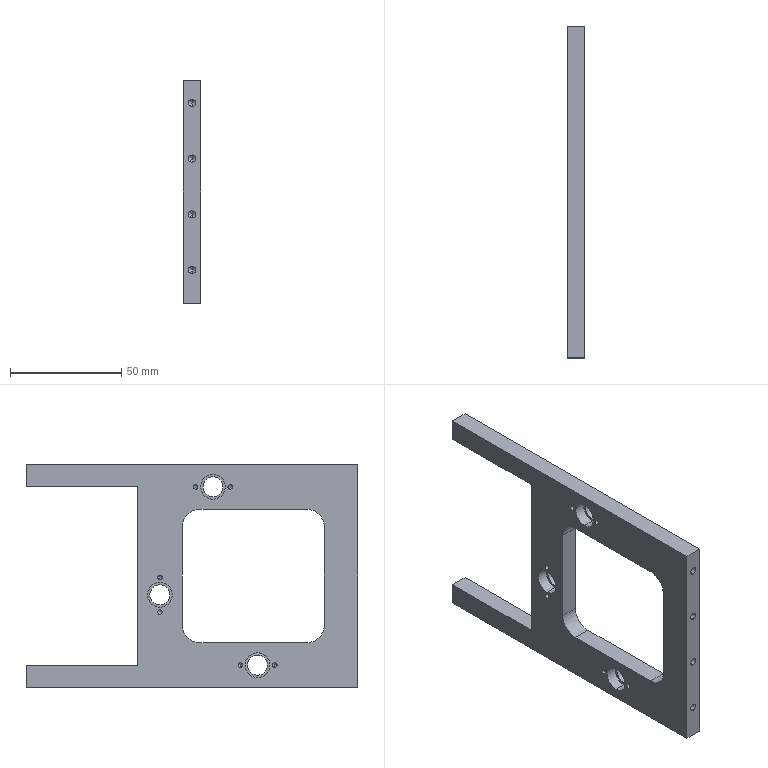Part | SolidWorks | features HoleWzd 4, ICE 3, 3DProfileFeature 1, Extrusion 1, Fillet 1 | 1 solid | 89 faces | box 8 x 148.83 x 100 mm | volume 54028 mm3 | cylinder 44 | cone 28 | plane 17 | commonest cylinder face diameters 3.3 x16 2.05 x12 9 x6 11.1 x6 16 x4